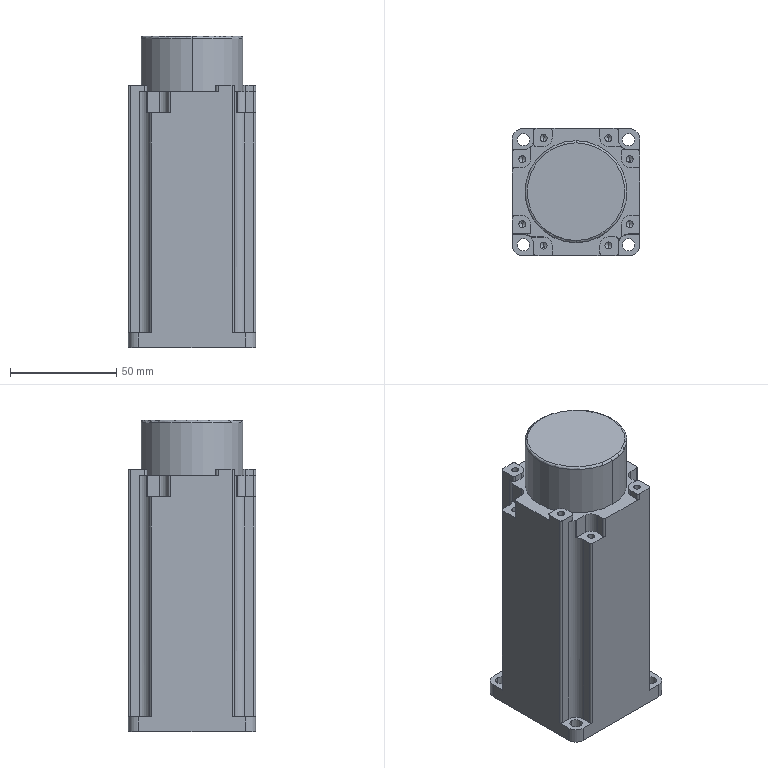Part | STEP file | Drive motor | 1 solid | 127 faces | box 60 x 60 x 146.5 mm | volume 432413 mm3 | cylinder 66 | plane 43 | cone 16 | torus 2 | commonest cylinder face diameters 2 x24 3.3 x16 5.8 x8 8 x8 9.8 x4 10 x4